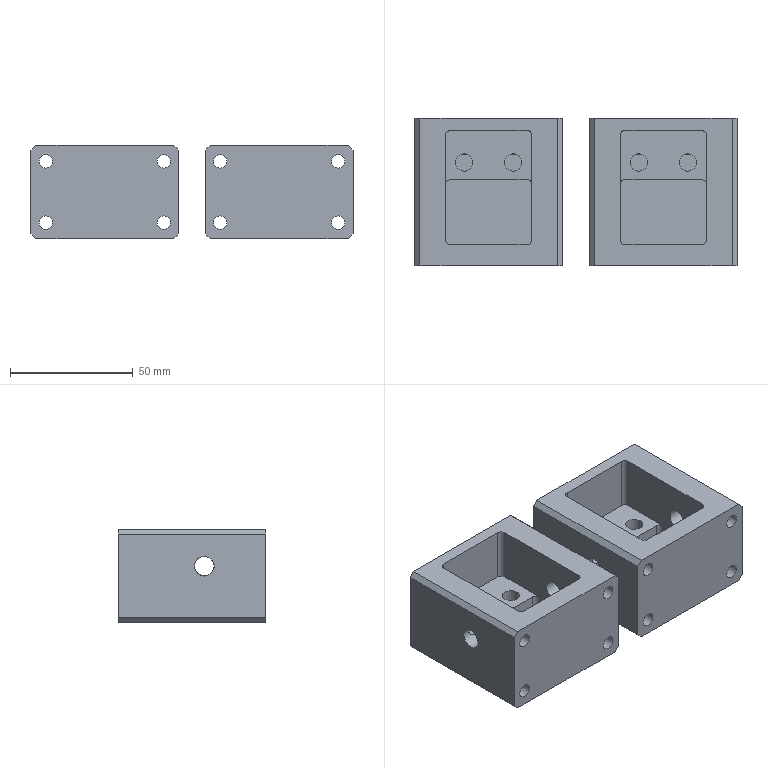Part | 2 solids | 94 faces | box 131 x 60 x 38 mm | volume 156649 mm3 | plane 50 | cylinder 44 | commonest cylinder face diameters 4 x12 5.5 x8 10 x8 4.2 x4 6 x4 7 x4